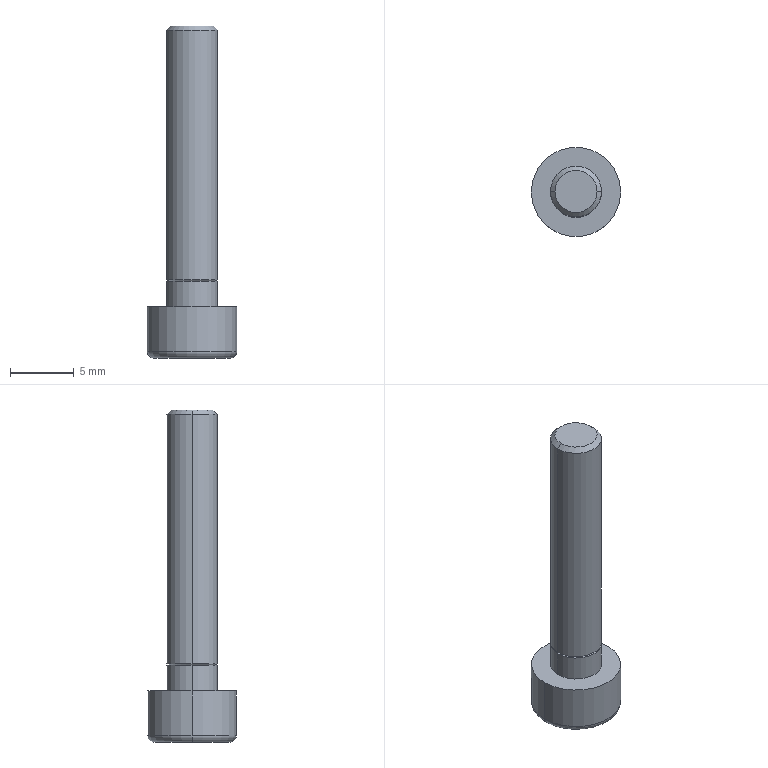Part | SolidWorks | features BaseBody 1 | 1 solid | 27 faces | box 7 x 7 x 26 mm | volume 416.594 mm3 | plane 11 | torus 6 | cylinder 6 | cone 4 | commonest cylinder face diameters 4 x4 7 x2
STEP:
#1=CARTESIAN_POINT('',(-1.763,0.,2.01));
#2=VERTEX_POINT('',#1);
#3=CARTESIAN_POINT('',(-1.743,0.,2.03));
#4=VERTEX_POINT('',#3);
#5=CARTESIAN_POINT('',(-1.763,0.,2.03));
#6=DIRECTION('',(0.,-1.,0.));
#7=DIRECTION('',(0.,0.,-1.));
#8=AXIS2_PLACEMENT_3D('',#5,#6,#7);
#9=CIRCLE('',#8,0.02);
#10=EDGE_CURVE('',#2,#4,#9,.T.);
#11=ORIENTED_EDGE('',*,*,#10,.T.);
#12=CARTESIAN_POINT('',(1.743,0.,2.03));
#13=VERTEX_POINT('',#12);
#14=CARTESIAN_POINT('',(0.,0.,2.03));
#15=DIRECTION('',(0.,0.,-1.));
#16=DIRECTION('',(-1.,0.,0.));
#17=AXIS2_PLACEMENT_3D('',#14,#15,#16);
#18=CIRCLE('',#17,1.743);
#19=EDGE_CURVE('',#4,#13,#18,.T.);
#20=ORIENTED_EDGE('',*,*,#19,.T.);
#21=CARTESIAN_POINT('',(1.763,0.,2.01));
#22=VERTEX_POINT('',#21);
#23=CARTESIAN_POINT('',(1.763,0.,2.03));
#24=DIRECTION('',(0.,1.,0.));
#25=DIRECTION('',(-1.,0.,0.));
#26=AXIS2_PLACEMENT_3D('',#23,#24,#25);
#27=CIRCLE('',#26,0.02);
#28=EDGE_CURVE('',#22,#13,#27,.T.);
#29=ORIENTED_EDGE('',*,*,#28,.F.);
#30=CARTESIAN_POINT('',(0.,0.,2.01));
#31=DIRECTION('',(0.,0.,-1.));
#32=DIRECTION('',(-1.,0.,0.));
#33=AXIS2_PLACEMENT_3D('',#30,#31,#32);
#34=CIRCLE('',#33,1.763);
#35=EDGE_CURVE('',#2,#22,#34,.T.);
#36=ORIENTED_EDGE('',*,*,#35,.F.);
#37=EDGE_LOOP('',(#11,#20,#29,#36));
#38=FACE_OUTER_BOUND('',#37,.T.);
#39=CARTESIAN_POINT('',(0.,0.,2.03));
#40=DIRECTION('',(0.,0.,-1.));
#41=DIRECTION('',(-1.,0.,0.));
#42=AXIS2_PLACEMENT_3D('',#39,#40,#41);
#43=TOROIDAL_SURFACE('',#42,1.763,0.02);
#44=ADVANCED_FACE('',(#38),#43,.F.);
#45=ORIENTED_EDGE('',*,*,#28,.T.);
#46=CARTESIAN_POINT('',(0.,0.,2.03));
#47=DIRECTION('',(0.,0.,-1.));
#48=DIRECTION('',(-1.,0.,0.));
#49=AXIS2_PLACEMENT_3D('',#46,#47,#48);
#50=CIRCLE('',#49,1.743);
#51=EDGE_CURVE('',#13,#4,#50,.T.);
#52=ORIENTED_EDGE('',*,*,#51,.T.);
#53=ORIENTED_EDGE('',*,*,#10,.F.);
#54=CARTESIAN_POINT('',(0.,0.,2.01));
#55=DIRECTION('',(0.,0.,-1.));
#56=DIRECTION('',(-1.,0.,0.));
#57=AXIS2_PLACEMENT_3D('',#54,#55,#56);
#58=CIRCLE('',#57,1.763);
#59=EDGE_CURVE('',#22,#2,#58,.T.);
#60=ORIENTED_EDGE('',*,*,#59,.F.);
#61=EDGE_LOOP('',(#45,#52,#53,#60));
#62=FACE_OUTER_BOUND('',#61,.T.);
#63=CARTESIAN_POINT('',(0.,0.,2.03));
#64=DIRECTION('',(0.,0.,-1.));
#65=DIRECTION('',(-1.,0.,0.));
#66=AXIS2_PLACEMENT_3D('',#63,#64,#65);
#67=TOROIDAL_SURFACE('',#66,1.763,0.02);
#68=ADVANCED_FACE('',(#62),#67,.F.);
#69=CARTESIAN_POINT('',(-1.65,0.,22.));
#70=VERTEX_POINT('',#69);
#71=CARTESIAN_POINT('',(1.65,0.,22.));
#72=VERTEX_POINT('',#71);
#73=CARTESIAN_POINT('',(0.,0.,22.));
#74=DIRECTION('',(0.,0.,-1.));
#75=DIRECTION('',(-1.,0.,0.));
#76=AXIS2_PLACEMENT_3D('',#73,#74,#75);
#77=CIRCLE('',#76,1.65);
#78=EDGE_CURVE('',#70,#72,#77,.T.);
#79=ORIENTED_EDGE('',*,*,#78,.T.);
#80=CARTESIAN_POINT('',(2.,0.,21.65));
#81=VERTEX_POINT('',#80);
#82=CARTESIAN_POINT('',(1.65,0.,22.));
#83=DIRECTION('',(0.7071,0.,-0.7071));
#84=VECTOR('',#83,1000.);
#85=LINE('',#82,#84);
#86=EDGE_CURVE('',#72,#81,#85,.T.);
#87=ORIENTED_EDGE('',*,*,#86,.T.);
#88=CARTESIAN_POINT('',(-2.,0.,21.65));
#89=VERTEX_POINT('',#88);
#90=CARTESIAN_POINT('',(0.,0.,21.65));
#91=DIRECTION('',(0.,0.,-1.));
#92=DIRECTION('',(-1.,0.,0.));
#93=AXIS2_PLACEMENT_3D('',#90,#91,#92);
#94=CIRCLE('',#93,2.);
#95=EDGE_CURVE('',#89,#81,#94,.T.);
#96=ORIENTED_EDGE('',*,*,#95,.F.);
#97=CARTESIAN_POINT('',(-1.65,0.,22.));
#98=DIRECTION('',(-0.7071,0.,-0.7071));
#99=VECTOR('',#98,1000.);
#100=LINE('',#97,#99);
#101=EDGE_CURVE('',#70,#89,#100,.T.);
#102=ORIENTED_EDGE('',*,*,#101,.F.);
#103=EDGE_LOOP('',(#79,#87,#96,#102));
#104=FACE_OUTER_BOUND('',#103,.T.);
#105=CARTESIAN_POINT('',(0.,0.,22.));
#106=DIRECTION('',(0.,0.,-1.));
#107=DIRECTION('',(-1.,0.,0.));
#108=AXIS2_PLACEMENT_3D('',#105,#106,#107);
#109=CONICAL_SURFACE('',#108,1.65,0.7854);
#110=ADVANCED_FACE('',(#104),#109,.T.);
#111=ORIENTED_EDGE('',*,*,#95,.T.);
#112=CARTESIAN_POINT('',(2.,0.,2.137));
#113=VERTEX_POINT('',#112);
#114=CARTESIAN_POINT('',(2.,0.,-10.585));
#115=DIRECTION('',(0.,0.,-1.));
#116=VECTOR('',#115,1000.);
#117=LINE('',#114,#116);
#118=EDGE_CURVE('',#81,#113,#117,.T.);
#119=ORIENTED_EDGE('',*,*,#118,.T.);
#120=CARTESIAN_POINT('',(-2.,0.,2.137));
#121=VERTEX_POINT('',#120);
#122=CARTESIAN_POINT('',(0.,0.,2.137));
#123=DIRECTION('',(0.,0.,-1.));
#124=DIRECTION('',(-1.,0.,0.));
#125=AXIS2_PLACEMENT_3D('',#122,#123,#124);
#126=CIRCLE('',#125,2.);
#127=EDGE_CURVE('',#121,#113,#126,.T.);
#128=ORIENTED_EDGE('',*,*,#127,.F.);
#129=CARTESIAN_POINT('',(-2.,0.,-10.585));
#130=DIRECTION('',(0.,0.,-1.));
#131=VECTOR('',#130,1000.);
#132=LINE('',#129,#131);
#133=EDGE_CURVE('',#89,#121,#132,.T.);
#134=ORIENTED_EDGE('',*,*,#133,.F.);
#135=EDGE_LOOP('',(#111,#119,#128,#134));
#136=FACE_OUTER_BOUND('',#135,.T.);
#137=CARTESIAN_POINT('',(0.,0.,-10.585));
#138=DIRECTION('',(0.,0.,-1.));
#139=DIRECTION('',(-1.,0.,0.));
#140=AXIS2_PLACEMENT_3D('',#137,#138,#139);
#141=CYLINDRICAL_SURFACE('',#140,2.);
#142=ADVANCED_FACE('',(#136),#141,.T.);
#143=CARTESIAN_POINT('',(-1.757,0.,2.049));
#144=VERTEX_POINT('',#143);
#145=CARTESIAN_POINT('',(1.757,0.,2.049));
#146=VERTEX_POINT('',#145);
#147=CARTESIAN_POINT('',(0.,0.,2.049));
#148=DIRECTION('',(0.,0.,-1.));
#149=DIRECTION('',(-1.,0.,0.));
#150=AXIS2_PLACEMENT_3D('',#147,#148,#149);
#151=CIRCLE('',#150,1.757);
#152=EDGE_CURVE('',#144,#146,#151,.T.);
#153=ORIENTED_EDGE('',*,*,#152,.F.);
#154=CARTESIAN_POINT('',(-2.,0.,2.137));
#155=DIRECTION('',(-0.9397,0.,0.342));
#156=VECTOR('',#155,1000.);
#157=LINE('',#154,#156);
#158=EDGE_CURVE('',#144,#121,#157,.T.);
#159=ORIENTED_EDGE('',*,*,#158,.T.);
#160=ORIENTED_EDGE('',*,*,#127,.T.);
#161=CARTESIAN_POINT('',(2.,0.,2.137));
#162=DIRECTION('',(0.9397,0.,0.342));
#163=VECTOR('',#162,1000.);
#164=LINE('',#161,#163);
#165=EDGE_CURVE('',#146,#113,#164,.T.);
#166=ORIENTED_EDGE('',*,*,#165,.F.);
#167=EDGE_LOOP('',(#153,#159,#160,#166));
#168=FACE_OUTER_BOUND('',#167,.T.);
#169=CARTESIAN_POINT('',(0.,0.,2.137));
#170=DIRECTION('',(0.,0.,1.));
#171=DIRECTION('',(1.,0.,0.));
#172=AXIS2_PLACEMENT_3D('',#169,#170,#171);
#173=CONICAL_SURFACE('',#172,2.,1.222);
#174=ADVANCED_FACE('',(#168),#173,.T.);
#175=ORIENTED_EDGE('',*,*,#51,.F.);
#176=CARTESIAN_POINT('',(1.763,0.,2.03));
#177=DIRECTION('',(0.,1.,0.));
#178=DIRECTION('',(-1.,0.,0.));
#179=AXIS2_PLACEMENT_3D('',#176,#177,#178);
#180=CIRCLE('',#179,0.02);
#181=EDGE_CURVE('',#13,#146,#180,.T.);
#182=ORIENTED_EDGE('',*,*,#181,.T.);
#183=CARTESIAN_POINT('',(0.,0.,2.049));
#184=DIRECTION('',(0.,0.,-1.));
#185=DIRECTION('',(-1.,0.,0.));
#186=AXIS2_PLACEMENT_3D('',#183,#184,#185);
#187=CIRCLE('',#186,1.757);
#188=EDGE_CURVE('',#146,#144,#187,.T.);
#189=ORIENTED_EDGE('',*,*,#188,.T.);
#190=CARTESIAN_POINT('',(-1.763,0.,2.03));
#191=DIRECTION('',(0.,-1.,0.));
#192=DIRECTION('',(0.,0.,-1.));
#193=AXIS2_PLACEMENT_3D('',#190,#191,#192);
#194=CIRCLE('',#193,0.02);
#195=EDGE_CURVE('',#4,#144,#194,.T.);
#196=ORIENTED_EDGE('',*,*,#195,.F.);
#197=EDGE_LOOP('',(#175,#182,#189,#196));
#198=FACE_OUTER_BOUND('',#197,.T.);
#199=CARTESIAN_POINT('',(0.,0.,2.03));
#200=DIRECTION('',(0.,0.,-1.));
#201=DIRECTION('',(-1.,0.,0.));
#202=AXIS2_PLACEMENT_3D('',#199,#200,#201);
#203=TOROIDAL_SURFACE('',#202,1.763,0.02);
#204=ADVANCED_FACE('',(#198),#203,.F.);
#205=CARTESIAN_POINT('',(-2.,0.,2.01));
#206=VERTEX_POINT('',#205);
#207=CARTESIAN_POINT('',(2.,0.,2.01));
#208=VERTEX_POINT('',#207);
#209=CARTESIAN_POINT('',(0.,0.,2.01));
#210=DIRECTION('',(0.,0.,-1.));
#211=DIRECTION('',(-1.,0.,0.));
#212=AXIS2_PLACEMENT_3D('',#209,#210,#211);
#213=CIRCLE('',#212,2.);
#214=EDGE_CURVE('',#206,#208,#213,.T.);
#215=ORIENTED_EDGE('',*,*,#214,.T.);
#216=CARTESIAN_POINT('',(2.,0.,0.));
#217=VERTEX_POINT('',#216);
#218=CARTESIAN_POINT('',(2.,0.,-10.585));
#219=DIRECTION('',(0.,0.,-1.));
#220=VECTOR('',#219,1000.);
#221=LINE('',#218,#220);
#222=EDGE_CURVE('',#208,#217,#221,.T.);
#223=ORIENTED_EDGE('',*,*,#222,.T.);
#224=CARTESIAN_POINT('',(-2.,0.,0.));
#225=VERTEX_POINT('',#224);
#226=CARTESIAN_POINT('',(0.,0.,0.));
#227=DIRECTION('',(0.,0.,-1.));
#228=DIRECTION('',(-1.,0.,0.));
#229=AXIS2_PLACEMENT_3D('',#226,#227,#228);
#230=CIRCLE('',#229,2.);
#231=EDGE_CURVE('',#225,#217,#230,.T.);
#232=ORIENTED_EDGE('',*,*,#231,.F.);
#233=CARTESIAN_POINT('',(-2.,0.,-10.585));
#234=DIRECTION('',(0.,0.,-1.));
#235=VECTOR('',#234,1000.);
#236=LINE('',#233,#235);
#237=EDGE_CURVE('',#206,#225,#236,.T.);
#238=ORIENTED_EDGE('',*,*,#237,.F.);
#239=EDGE_LOOP('',(#215,#223,#232,#238));
#240=FACE_OUTER_BOUND('',#239,.T.);
#241=CARTESIAN_POINT('',(0.,0.,-10.585));
#242=DIRECTION('',(0.,0.,-1.));
#243=DIRECTION('',(-1.,0.,0.));
#244=AXIS2_PLACEMENT_3D('',#241,#242,#243);
#245=CYLINDRICAL_SURFACE('',#244,2.);
#246=ADVANCED_FACE('',(#240),#245,.T.);
#247=CARTESIAN_POINT('',(-3.5,0.,0.));
#248=VERTEX_POINT('',#247);
#249=CARTESIAN_POINT('',(3.5,0.,0.));
#250=VERTEX_POINT('',#249);
#251=CARTESIAN_POINT('',(0.,0.,0.));
#252=DIRECTION('',(0.,0.,-1.));
#253=DIRECTION('',(-1.,0.,0.));
#254=AXIS2_PLACEMENT_3D('',#251,#252,#253);
#255=CIRCLE('',#254,3.5);
#256=EDGE_CURVE('',#248,#250,#255,.T.);
#257=ORIENTED_EDGE('',*,*,#256,.T.);
#258=CARTESIAN_POINT('',(3.5,0.,-3.5));
#259=VERTEX_POINT('',#258);
#260=CARTESIAN_POINT('',(3.5,0.,-10.585));
#261=DIRECTION('',(0.,0.,-1.));
#262=VECTOR('',#261,1000.);
#263=LINE('',#260,#262);
#264=EDGE_CURVE('',#250,#259,#263,.T.);
#265=ORIENTED_EDGE('',*,*,#264,.T.);
#266=CARTESIAN_POINT('',(-3.5,0.,-3.5));
#267=VERTEX_POINT('',#266);
#268=CARTESIAN_POINT('',(0.,0.,-3.5));
#269=DIRECTION('',(0.,0.,-1.));
#270=DIRECTION('',(-1.,0.,0.));
#271=AXIS2_PLACEMENT_3D('',#268,#269,#270);
#272=CIRCLE('',#271,3.5);
#273=EDGE_CURVE('',#267,#259,#272,.T.);
#274=ORIENTED_EDGE('',*,*,#273,.F.);
#275=CARTESIAN_POINT('',(-3.5,0.,-10.585));
#276=DIRECTION('',(0.,0.,-1.));
#277=VECTOR('',#276,1000.);
#278=LINE('',#275,#277);
#279=EDGE_CURVE('',#248,#267,#278,.T.);
#280=ORIENTED_EDGE('',*,*,#279,.F.);
#281=EDGE_LOOP('',(#257,#265,#274,#280));
#282=FACE_OUTER_BOUND('',#281,.T.);
#283=CARTESIAN_POINT('',(0.,0.,-10.585));
#284=DIRECTION('',(0.,0.,-1.));
#285=DIRECTION('',(-1.,0.,0.));
#286=AXIS2_PLACEMENT_3D('',#283,#284,#285);
#287=CYLINDRICAL_SURFACE('',#286,3.5);
#288=ADVANCED_FACE('',(#282),#287,.T.);
#289=ORIENTED_EDGE('',*,*,#273,.T.);
#290=CARTESIAN_POINT('',(3.,0.,-4.));
#291=VERTEX_POINT('',#290);
#292=CARTESIAN_POINT('',(3.,0.,-3.5));
#293=DIRECTION('',(0.,1.,0.));
#294=DIRECTION('',(-1.,0.,0.));
#295=AXIS2_PLACEMENT_3D('',#292,#293,#294);
#296=CIRCLE('',#295,0.5);
#297=EDGE_CURVE('',#259,#291,#296,.T.);
#298=ORIENTED_EDGE('',*,*,#297,.T.);
#299=CARTESIAN_POINT('',(-3.,0.,-4.));
#300=VERTEX_POINT('',#299);
#301=CARTESIAN_POINT('',(0.,0.,-4.));
#302=DIRECTION('',(0.,0.,-1.));
#303=DIRECTION('',(-1.,0.,0.));
#304=AXIS2_PLACEMENT_3D('',#301,#302,#303);
#305=CIRCLE('',#304,3.);
#306=EDGE_CURVE('',#300,#291,#305,.T.);
#307=ORIENTED_EDGE('',*,*,#306,.F.);
#308=CARTESIAN_POINT('',(-3.,0.,-3.5));
#309=DIRECTION('',(0.,-1.,0.));
#310=DIRECTION('',(0.,0.,-1.));
#311=AXIS2_PLACEMENT_3D('',#308,#309,#310);
#312=CIRCLE('',#311,0.5);
#313=EDGE_CURVE('',#267,#300,#312,.T.);
#314=ORIENTED_EDGE('',*,*,#313,.F.);
#315=EDGE_LOOP('',(#289,#298,#307,#314));
#316=FACE_OUTER_BOUND('',#315,.T.);
#317=CARTESIAN_POINT('',(0.,0.,-3.5));
#318=DIRECTION('',(0.,0.,-1.));
#319=DIRECTION('',(-1.,0.,0.));
#320=AXIS2_PLACEMENT_3D('',#317,#318,#319);
#321=TOROIDAL_SURFACE('',#320,3.,0.5);
#322=ADVANCED_FACE('',(#316),#321,.T.);
#323=ORIENTED_EDGE('',*,*,#297,.F.);
#324=CARTESIAN_POINT('',(0.,0.,-3.5));
#325=DIRECTION('',(0.,0.,-1.));
#326=DIRECTION('',(-1.,0.,0.));
#327=AXIS2_PLACEMENT_3D('',#324,#325,#326);
#328=CIRCLE('',#327,3.5);
#329=EDGE_CURVE('',#259,#267,#328,.T.);
#330=ORIENTED_EDGE('',*,*,#329,.T.);
#331=ORIENTED_EDGE('',*,*,#313,.T.);
#332=CARTESIAN_POINT('',(0.,0.,-4.));
#333=DIRECTION('',(0.,0.,-1.));
#334=DIRECTION('',(-1.,0.,0.));
#335=AXIS2_PLACEMENT_3D('',#332,#333,#334);
#336=CIRCLE('',#335,3.);
#337=EDGE_CURVE('',#291,#300,#336,.T.);
#338=ORIENTED_EDGE('',*,*,#337,.F.);
#339=EDGE_LOOP('',(#323,#330,#331,#338));
#340=FACE_OUTER_BOUND('',#339,.T.);
#341=CARTESIAN_POINT('',(0.,0.,-3.5));
#342=DIRECTION('',(0.,0.,-1.));
#343=DIRECTION('',(-1.,0.,0.));
#344=AXIS2_PLACEMENT_3D('',#341,#342,#343);
#345=TOROIDAL_SURFACE('',#344,3.,0.5);
#346=ADVANCED_FACE('',(#340),#345,.T.);
#347=ORIENTED_EDGE('',*,*,#264,.F.);
#348=CARTESIAN_POINT('',(0.,0.,0.));
#349=DIRECTION('',(0.,0.,-1.));
#350=DIRECTION('',(-1.,0.,0.));
#351=AXIS2_PLACEMENT_3D('',#348,#349,#350);
#352=CIRCLE('',#351,3.5);
#353=EDGE_CURVE('',#250,#248,#352,.T.);
#354=ORIENTED_EDGE('',*,*,#353,.T.);
#355=ORIENTED_EDGE('',*,*,#279,.T.);
#356=ORIENTED_EDGE('',*,*,#329,.F.);
#357=EDGE_LOOP('',(#347,#354,#355,#356));
#358=FACE_OUTER_BOUND('',#357,.T.);
#359=CARTESIAN_POINT('',(0.,0.,-10.585));
#360=DIRECTION('',(0.,0.,-1.));
#361=DIRECTION('',(-1.,0.,0.));
#362=AXIS2_PLACEMENT_3D('',#359,#360,#361);
#363=CYLINDRICAL_SURFACE('',#362,3.5);
#364=ADVANCED_FACE('',(#358),#363,.T.);
#365=ORIENTED_EDGE('',*,*,#256,.F.);
#366=ORIENTED_EDGE('',*,*,#353,.F.);
#367=EDGE_LOOP('',(#365,#366));
#368=FACE_OUTER_BOUND('',#367,.T.);
#369=ORIENTED_EDGE('',*,*,#231,.T.);
#370=CARTESIAN_POINT('',(0.,0.,0.));
#371=DIRECTION('',(0.,0.,-1.));
#372=DIRECTION('',(-1.,0.,0.));
#373=AXIS2_PLACEMENT_3D('',#370,#371,#372);
#374=CIRCLE('',#373,2.);
#375=EDGE_CURVE('',#217,#225,#374,.T.);
#376=ORIENTED_EDGE('',*,*,#375,.T.);
#377=EDGE_LOOP('',(#369,#376));
#378=FACE_BOUND('',#377,.T.);
#379=CARTESIAN_POINT('',(-3.5,0.,0.));
#380=DIRECTION('',(0.,0.,-1.));
#381=DIRECTION('',(-1.,0.,0.));
#382=AXIS2_PLACEMENT_3D('',#379,#380,#381);
#383=PLANE('',#382);
#384=ADVANCED_FACE('',(#368,#378),#383,.F.);
#385=ORIENTED_EDGE('',*,*,#222,.F.);
#386=CARTESIAN_POINT('',(0.,0.,2.01));
#387=DIRECTION('',(0.,0.,-1.));
#388=DIRECTION('',(-1.,0.,0.));
#389=AXIS2_PLACEMENT_3D('',#386,#387,#388);
#390=CIRCLE('',#389,2.);
#391=EDGE_CURVE('',#208,#206,#390,.T.);
#392=ORIENTED_EDGE('',*,*,#391,.T.);
#393=ORIENTED_EDGE('',*,*,#237,.T.);
#394=ORIENTED_EDGE('',*,*,#375,.F.);
#395=EDGE_LOOP('',(#385,#392,#393,#394));
#396=FACE_OUTER_BOUND('',#395,.T.);
#397=CARTESIAN_POINT('',(0.,0.,-10.585));
#398=DIRECTION('',(0.,0.,-1.));
#399=DIRECTION('',(-1.,0.,0.));
#400=AXIS2_PLACEMENT_3D('',#397,#398,#399);
#401=CYLINDRICAL_SURFACE('',#400,2.);
#402=ADVANCED_FACE('',(#396),#401,.T.);
#403=ORIENTED_EDGE('',*,*,#214,.F.);
#404=ORIENTED_EDGE('',*,*,#391,.F.);
#405=EDGE_LOOP('',(#403,#404));
#406=FACE_OUTER_BOUND('',#405,.T.);
#407=ORIENTED_EDGE('',*,*,#35,.T.);
#408=ORIENTED_EDGE('',*,*,#59,.T.);
#409=EDGE_LOOP('',(#407,#408));
#410=FACE_BOUND('',#409,.T.);
#411=CARTESIAN_POINT('',(-2.,0.,2.01));
#412=DIRECTION('',(0.,0.,-1.));
#413=DIRECTION('',(-1.,0.,0.));
#414=AXIS2_PLACEMENT_3D('',#411,#412,#413);
#415=PLANE('',#414);
#416=ADVANCED_FACE('',(#406,#410),#415,.F.);
#417=ORIENTED_EDGE('',*,*,#19,.F.);
#418=ORIENTED_EDGE('',*,*,#195,.T.);
#419=ORIENTED_EDGE('',*,*,#152,.T.);
#420=ORIENTED_EDGE('',*,*,#181,.F.);
#421=EDGE_LOOP('',(#417,#418,#419,#420));
#422=FACE_OUTER_BOUND('',#421,.T.);
#423=CARTESIAN_POINT('',(0.,0.,2.03));
#424=DIRECTION('',(0.,0.,-1.));
#425=DIRECTION('',(-1.,0.,0.));
#426=AXIS2_PLACEMENT_3D('',#423,#424,#425);
#427=TOROIDAL_SURFACE('',#426,1.763,0.02);
#428=ADVANCED_FACE('',(#422),#427,.F.);
#429=ORIENTED_EDGE('',*,*,#158,.F.);
#430=ORIENTED_EDGE('',*,*,#188,.F.);
#431=ORIENTED_EDGE('',*,*,#165,.T.);
#432=CARTESIAN_POINT('',(0.,0.,2.137));
#433=DIRECTION('',(0.,0.,-1.));
#434=DIRECTION('',(-1.,0.,0.));
#435=AXIS2_PLACEMENT_3D('',#432,#433,#434);
#436=CIRCLE('',#435,2.);
#437=EDGE_CURVE('',#113,#121,#436,.T.);
#438=ORIENTED_EDGE('',*,*,#437,.T.);
#439=EDGE_LOOP('',(#429,#430,#431,#438));
#440=FACE_OUTER_BOUND('',#439,.T.);
#441=CARTESIAN_POINT('',(0.,0.,2.137));
#442=DIRECTION('',(0.,0.,1.));
#443=DIRECTION('',(1.,0.,0.));
#444=AXIS2_PLACEMENT_3D('',#441,#442,#443);
#445=CONICAL_SURFACE('',#444,2.,1.222);
#446=ADVANCED_FACE('',(#440),#445,.T.);
#447=ORIENTED_EDGE('',*,*,#118,.F.);
#448=CARTESIAN_POINT('',(0.,0.,21.65));
#449=DIRECTION('',(0.,0.,-1.));
#450=DIRECTION('',(-1.,0.,0.));
#451=AXIS2_PLACEMENT_3D('',#448,#449,#450);
#452=CIRCLE('',#451,2.);
#453=EDGE_CURVE('',#81,#89,#452,.T.);
#454=ORIENTED_EDGE('',*,*,#453,.T.);
#455=ORIENTED_EDGE('',*,*,#133,.T.);
#456=ORIENTED_EDGE('',*,*,#437,.F.);
#457=EDGE_LOOP('',(#447,#454,#455,#456));
#458=FACE_OUTER_BOUND('',#457,.T.);
#459=CARTESIAN_POINT('',(0.,0.,-10.585));
#460=DIRECTION('',(0.,0.,-1.));
#461=DIRECTION('',(-1.,0.,0.));
#462=AXIS2_PLACEMENT_3D('',#459,#460,#461);
#463=CYLINDRICAL_SURFACE('',#462,2.);
#464=ADVANCED_FACE('',(#458),#463,.T.);
#465=ORIENTED_EDGE('',*,*,#86,.F.);
#466=CARTESIAN_POINT('',(0.,0.,22.));
#467=DIRECTION('',(0.,0.,-1.));
#468=DIRECTION('',(-1.,0.,0.));
#469=AXIS2_PLACEMENT_3D('',#466,#467,#468);
#470=CIRCLE('',#469,1.65);
#471=EDGE_CURVE('',#72,#70,#470,.T.);
#472=ORIENTED_EDGE('',*,*,#471,.T.);
#473=ORIENTED_EDGE('',*,*,#101,.T.);
#474=ORIENTED_EDGE('',*,*,#453,.F.);
#475=EDGE_LOOP('',(#465,#472,#473,#474));
#476=FACE_OUTER_BOUND('',#475,.T.);
#477=CARTESIAN_POINT('',(0.,0.,22.));
#478=DIRECTION('',(0.,0.,-1.));
#479=DIRECTION('',(-1.,0.,0.));
#480=AXIS2_PLACEMENT_3D('',#477,#478,#479);
#481=CONICAL_SURFACE('',#480,1.65,0.7854);
#482=ADVANCED_FACE('',(#476),#481,.T.);
#483=ORIENTED_EDGE('',*,*,#78,.F.);
#484=ORIENTED_EDGE('',*,*,#471,.F.);
#485=EDGE_LOOP('',(#483,#484));
#486=FACE_OUTER_BOUND('',#485,.T.);
#487=CARTESIAN_POINT('',(-1.65,0.,22.));
#488=DIRECTION('',(0.,0.,-1.));
#489=DIRECTION('',(-1.,0.,0.));
#490=AXIS2_PLACEMENT_3D('',#487,#488,#489);
#491=PLANE('',#490);
#492=ADVANCED_FACE('',(#486),#491,.F.);
#493=CARTESIAN_POINT('',(1.732,0.,-4.));
#494=VERTEX_POINT('',#493);
#495=CARTESIAN_POINT('',(0.866,-1.5,-4.));
#496=VERTEX_POINT('',#495);
#497=CARTESIAN_POINT('',(1.732,0.,-4.));
#498=DIRECTION('',(-0.5,-0.866,0.));
#499=VECTOR('',#498,1000.);
#500=LINE('',#497,#499);
#501=EDGE_CURVE('',#494,#496,#500,.T.);
#502=ORIENTED_EDGE('',*,*,#501,.F.);
#503=CARTESIAN_POINT('',(0.866,1.5,-4.));
#504=VERTEX_POINT('',#503);
#505=CARTESIAN_POINT('',(0.866,1.5,-4.));
#506=DIRECTION('',(0.5,-0.866,0.));
#507=VECTOR('',#506,1000.);
#508=LINE('',#505,#507);
#509=EDGE_CURVE('',#504,#494,#508,.T.);
#510=ORIENTED_EDGE('',*,*,#509,.F.);
#511=CARTESIAN_POINT('',(-0.866,1.5,-4.));
#512=VERTEX_POINT('',#511);
#513=CARTESIAN_POINT('',(-0.866,1.5,-4.));
#514=DIRECTION('',(1.,0.,0.));
#515=VECTOR('',#514,1000.);
#516=LINE('',#513,#515);
#517=EDGE_CURVE('',#512,#504,#516,.T.);
#518=ORIENTED_EDGE('',*,*,#517,.F.);
#519=CARTESIAN_POINT('',(-1.732,0.,-4.));
#520=VERTEX_POINT('',#519);
#521=CARTESIAN_POINT('',(-1.732,0.,-4.));
#522=DIRECTION('',(0.5,0.866,0.));
#523=VECTOR('',#522,1000.);
#524=LINE('',#521,#523);
#525=EDGE_CURVE('',#520,#512,#524,.T.);
#526=ORIENTED_EDGE('',*,*,#525,.F.);
#527=CARTESIAN_POINT('',(-0.866,-1.5,-4.));
#528=VERTEX_POINT('',#527);
#529=CARTESIAN_POINT('',(-0.866,-1.5,-4.));
#530=DIRECTION('',(-0.5,0.866,0.));
#531=VECTOR('',#530,1000.);
#532=LINE('',#529,#531);
#533=EDGE_CURVE('',#528,#520,#532,.T.);
#534=ORIENTED_EDGE('',*,*,#533,.F.);
#535=CARTESIAN_POINT('',(0.866,-1.5,-4.));
#536=DIRECTION('',(-1.,0.,0.));
#537=VECTOR('',#536,1000.);
#538=LINE('',#535,#537);
#539=EDGE_CURVE('',#496,#528,#538,.T.);
#540=ORIENTED_EDGE('',*,*,#539,.F.);
#541=EDGE_LOOP('',(#502,#510,#518,#526,#534,#540));
#542=FACE_BOUND('',#541,.T.);
#543=ORIENTED_EDGE('',*,*,#306,.T.);
#544=ORIENTED_EDGE('',*,*,#337,.T.);
#545=EDGE_LOOP('',(#543,#544));
#546=FACE_OUTER_BOUND('',#545,.T.);
#547=CARTESIAN_POINT('',(0.,0.,-4.));
#548=DIRECTION('',(0.,0.,1.));
#549=DIRECTION('',(1.,0.,0.));
#550=AXIS2_PLACEMENT_3D('',#547,#548,#549);
#551=PLANE('',#550);
#552=ADVANCED_FACE('',(#542,#546),#551,.F.);
#553=ORIENTED_EDGE('',*,*,#509,.T.);
#554=CARTESIAN_POINT('',(1.732,0.,-2.5));
#555=VERTEX_POINT('',#554);
#556=CARTESIAN_POINT('',(1.732,0.,-2.5));
#557=DIRECTION('',(0.,0.,-1.));
#558=VECTOR('',#557,1000.);
#559=LINE('',#556,#558);
#560=EDGE_CURVE('',#555,#494,#559,.T.);
#561=ORIENTED_EDGE('',*,*,#560,.F.);
#562=CARTESIAN_POINT('',(0.866,1.5,-2.5));
#563=VERTEX_POINT('',#562);
#564=CARTESIAN_POINT('',(0.866,1.5,-2.5));
#565=DIRECTION('',(0.5,-0.866,0.));
#566=VECTOR('',#565,1000.);
#567=LINE('',#564,#566);
#568=EDGE_CURVE('',#563,#555,#567,.T.);
#569=ORIENTED_EDGE('',*,*,#568,.F.);
#570=CARTESIAN_POINT('',(0.866,1.5,-2.5));
#571=DIRECTION('',(0.,0.,-1.));
#572=VECTOR('',#571,1000.);
#573=LINE('',#570,#572);
#574=EDGE_CURVE('',#563,#504,#573,.T.);
#575=ORIENTED_EDGE('',*,*,#574,.T.);
#576=EDGE_LOOP('',(#553,#561,#569,#575));
#577=FACE_OUTER_BOUND('',#576,.T.);
#578=CARTESIAN_POINT('',(0.866,1.5,-2.5));
#579=DIRECTION('',(0.866,0.5,0.));
#580=DIRECTION('',(-0.5,0.866,0.));
#581=AXIS2_PLACEMENT_3D('',#578,#579,#580);
#582=PLANE('',#581);
#583=ADVANCED_FACE('',(#577),#582,.F.);
#584=ORIENTED_EDGE('',*,*,#517,.T.);
#585=ORIENTED_EDGE('',*,*,#574,.F.);
#586=CARTESIAN_POINT('',(-0.866,1.5,-2.5));
#587=VERTEX_POINT('',#586);
#588=CARTESIAN_POINT('',(-0.866,1.5,-2.5));
#589=DIRECTION('',(1.,0.,0.));
#590=VECTOR('',#589,1000.);
#591=LINE('',#588,#590);
#592=EDGE_CURVE('',#587,#563,#591,.T.);
#593=ORIENTED_EDGE('',*,*,#592,.F.);
#594=CARTESIAN_POINT('',(-0.866,1.5,-2.5));
#595=DIRECTION('',(0.,0.,-1.));
#596=VECTOR('',#595,1000.);
#597=LINE('',#594,#596);
#598=EDGE_CURVE('',#587,#512,#597,.T.);
#599=ORIENTED_EDGE('',*,*,#598,.T.);
#600=EDGE_LOOP('',(#584,#585,#593,#599));
#601=FACE_OUTER_BOUND('',#600,.T.);
#602=CARTESIAN_POINT('',(-0.866,1.5,-2.5));
#603=DIRECTION('',(0.,1.,0.));
#604=DIRECTION('',(0.,0.,1.));
#605=AXIS2_PLACEMENT_3D('',#602,#603,#604);
#606=PLANE('',#605);
#607=ADVANCED_FACE('',(#601),#606,.F.);
#608=ORIENTED_EDGE('',*,*,#525,.T.);
#609=ORIENTED_EDGE('',*,*,#598,.F.);
#610=CARTESIAN_POINT('',(-1.732,0.,-2.5));
#611=VERTEX_POINT('',#610);
#612=CARTESIAN_POINT('',(-1.732,0.,-2.5));
#613=DIRECTION('',(0.5,0.866,0.));
#614=VECTOR('',#613,1000.);
#615=LINE('',#612,#614);
#616=EDGE_CURVE('',#611,#587,#615,.T.);
#617=ORIENTED_EDGE('',*,*,#616,.F.);
#618=CARTESIAN_POINT('',(-1.732,0.,-2.5));
#619=DIRECTION('',(0.,0.,-1.));
#620=VECTOR('',#619,1000.);
#621=LINE('',#618,#620);
#622=EDGE_CURVE('',#611,#520,#621,.T.);
#623=ORIENTED_EDGE('',*,*,#622,.T.);
#624=EDGE_LOOP('',(#608,#609,#617,#623));
#625=FACE_OUTER_BOUND('',#624,.T.);
#626=CARTESIAN_POINT('',(-1.732,0.,-2.5));
#627=DIRECTION('',(-0.866,0.5,0.));
#628=DIRECTION('',(-0.5,-0.866,0.));
#629=AXIS2_PLACEMENT_3D('',#626,#627,#628);
#630=PLANE('',#629);
#631=ADVANCED_FACE('',(#625),#630,.F.);
#632=ORIENTED_EDGE('',*,*,#533,.T.);
#633=ORIENTED_EDGE('',*,*,#622,.F.);
#634=CARTESIAN_POINT('',(-0.866,-1.5,-2.5));
#635=VERTEX_POINT('',#634);
#636=CARTESIAN_POINT('',(-0.866,-1.5,-2.5));
#637=DIRECTION('',(-0.5,0.866,0.));
#638=VECTOR('',#637,1000.);
#639=LINE('',#636,#638);
#640=EDGE_CURVE('',#635,#611,#639,.T.);
#641=ORIENTED_EDGE('',*,*,#640,.F.);
#642=CARTESIAN_POINT('',(-0.866,-1.5,-2.5));
#643=DIRECTION('',(0.,0.,-1.));
#644=VECTOR('',#643,1000.);
#645=LINE('',#642,#644);
#646=EDGE_CURVE('',#635,#528,#645,.T.);
#647=ORIENTED_EDGE('',*,*,#646,.T.);
#648=EDGE_LOOP('',(#632,#633,#641,#647));
#649=FACE_OUTER_BOUND('',#648,.T.);
#650=CARTESIAN_POINT('',(-0.866,-1.5,-2.5));
#651=DIRECTION('',(-0.866,-0.5,0.));
#652=DIRECTION('',(0.5,-0.866,0.));
#653=AXIS2_PLACEMENT_3D('',#650,#651,#652);
#654=PLANE('',#653);
#655=ADVANCED_FACE('',(#649),#654,.F.);
#656=ORIENTED_EDGE('',*,*,#539,.T.);
#657=ORIENTED_EDGE('',*,*,#646,.F.);
#658=CARTESIAN_POINT('',(0.866,-1.5,-2.5));
#659=VERTEX_POINT('',#658);
#660=CARTESIAN_POINT('',(0.866,-1.5,-2.5));
#661=DIRECTION('',(-1.,0.,0.));
#662=VECTOR('',#661,1000.);
#663=LINE('',#660,#662);
#664=EDGE_CURVE('',#659,#635,#663,.T.);
#665=ORIENTED_EDGE('',*,*,#664,.F.);
#666=CARTESIAN_POINT('',(0.866,-1.5,-2.5));
#667=DIRECTION('',(0.,0.,-1.));
#668=VECTOR('',#667,1000.);
#669=LINE('',#666,#668);
#670=EDGE_CURVE('',#659,#496,#669,.T.);
#671=ORIENTED_EDGE('',*,*,#670,.T.);
#672=EDGE_LOOP('',(#656,#657,#665,#671));
#673=FACE_OUTER_BOUND('',#672,.T.);
#674=CARTESIAN_POINT('',(0.866,-1.5,-2.5));
#675=DIRECTION('',(0.,-1.,0.));
#676=DIRECTION('',(0.,0.,-1.));
#677=AXIS2_PLACEMENT_3D('',#674,#675,#676);
#678=PLANE('',#677);
#679=ADVANCED_FACE('',(#673),#678,.F.);
#680=ORIENTED_EDGE('',*,*,#501,.T.);
#681=ORIENTED_EDGE('',*,*,#670,.F.);
#682=CARTESIAN_POINT('',(1.732,0.,-2.5));
#683=DIRECTION('',(-0.5,-0.866,0.));
#684=VECTOR('',#683,1000.);
#685=LINE('',#682,#684);
#686=EDGE_CURVE('',#555,#659,#685,.T.);
#687=ORIENTED_EDGE('',*,*,#686,.F.);
#688=ORIENTED_EDGE('',*,*,#560,.T.);
#689=EDGE_LOOP('',(#680,#681,#687,#688));
#690=FACE_OUTER_BOUND('',#689,.T.);
#691=CARTESIAN_POINT('',(1.732,0.,-2.5));
#692=DIRECTION('',(0.866,-0.5,0.));
#693=DIRECTION('',(0.5,0.866,0.));
#694=AXIS2_PLACEMENT_3D('',#691,#692,#693);
#695=PLANE('',#694);
#696=ADVANCED_FACE('',(#690),#695,.F.);
#697=ORIENTED_EDGE('',*,*,#568,.T.);
#698=ORIENTED_EDGE('',*,*,#686,.T.);
#699=ORIENTED_EDGE('',*,*,#664,.T.);
#700=ORIENTED_EDGE('',*,*,#640,.T.);
#701=ORIENTED_EDGE('',*,*,#616,.T.);
#702=ORIENTED_EDGE('',*,*,#592,.T.);
#703=EDGE_LOOP('',(#697,#698,#699,#700,#701,#702));
#704=FACE_OUTER_BOUND('',#703,.T.);
#705=CARTESIAN_POINT('',(0.866,1.5,-2.5));
#706=DIRECTION('',(0.,0.,1.));
#707=DIRECTION('',(1.,0.,0.));
#708=AXIS2_PLACEMENT_3D('',#705,#706,#707);
#709=PLANE('',#708);
#710=ADVANCED_FACE('',(#704),#709,.F.);
#711=CLOSED_SHELL('',(#44,#68,#110,#142,#174,#204,#246,#288,#322,#346,#364,#384,#402,#416,#428,#446,#464,#482,#492,#552,#583,#607,#631,#655,#679,#696,#710));
#712=MANIFOLD_SOLID_BREP('',#711);
#713=CARTESIAN_POINT('',(0.,0.,0.));
#714=DIRECTION('',(0.,0.,1.));
#715=DIRECTION('',(1.,0.,0.));
#716=AXIS2_PLACEMENT_3D('',#713,#714,#715);
#717=(LENGTH_UNIT()NAMED_UNIT(*)SI_UNIT(.MILLI.,.METRE.));
#718=UNCERTAINTY_MEASURE_WITH_UNIT(LENGTH_MEASURE(0.00001),#717,'','');
#719=(NAMED_UNIT(*)PLANE_ANGLE_UNIT()SI_UNIT($,.RADIAN.));
#720=(NAMED_UNIT(*)SI_UNIT($,.STERADIAN.)SOLID_ANGLE_UNIT());
#721=(GEOMETRIC_REPRESENTATION_CONTEXT(3)GLOBAL_UNCERTAINTY_ASSIGNED_CONTEXT((#718))GLOBAL_UNIT_ASSIGNED_CONTEXT((#717,#719,#720))REPRESENTATION_CONTEXT('',''));
#722=ADVANCED_BREP_SHAPE_REPRESENTATION('',(#712,#716),#721);